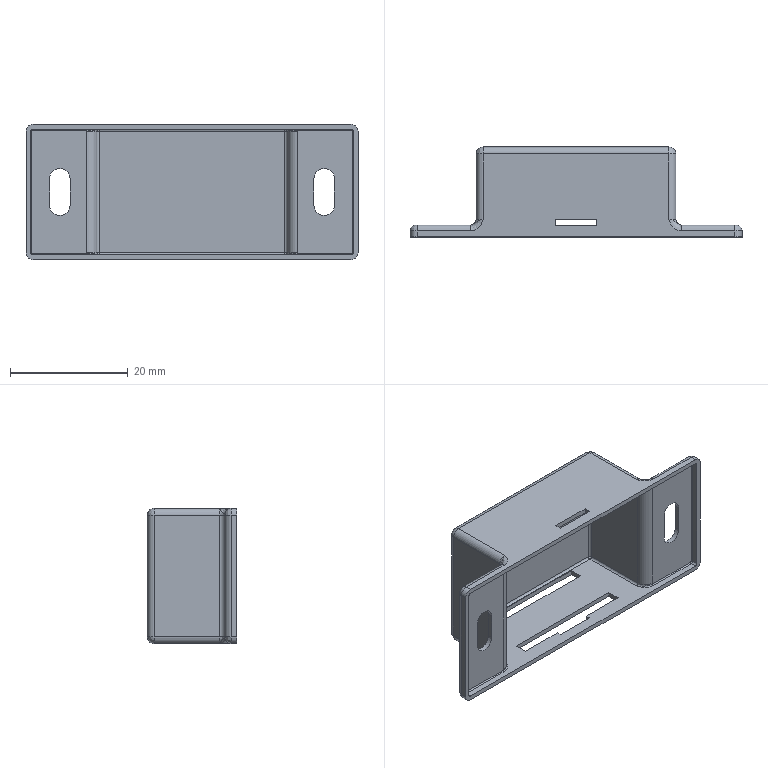Part | STEP file | Second C-100-B-2 Base Part | 1 solid | 115 faces | box 56.5 x 15.3 x 23 mm | volume 2154 mm3 | cylinder 44 | plane 39 | spline 32 | commonest cylinder face diameters 0.8 x12 2.4 x12 2 x8 0.4 x6 3.5 x4 3.6 x2